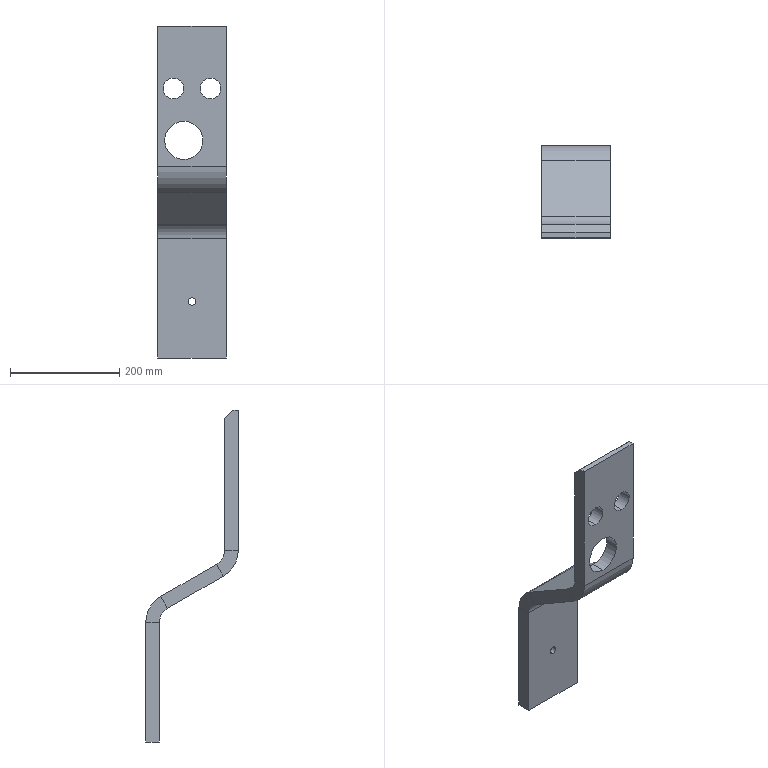Part | SolidWorks | features Chamfer 1, FlatPattern 1, HoleWzd 1, ICE 1, SMBaseFlange 1, SheetMetal 1 | 1 solid | 31 faces | box 126 x 169.5 x 608 mm | volume 1978271 mm3 | plane 19 | cylinder 12 | commonest cylinder face diameters 38 x4 14 x2 60 x2 70 x2 110 x2
STEP:
#1=CARTESIAN_POINT('',(0.,144.5,-397.));
#2=VERTEX_POINT('',#1);
#3=CARTESIAN_POINT('',(0.,144.5,-383.));
#4=VERTEX_POINT('',#3);
#5=CARTESIAN_POINT('',(0.,144.5,-390.));
#6=DIRECTION('',(0.,1.,0.));
#7=DIRECTION('',(0.,0.,1.));
#8=AXIS2_PLACEMENT_3D('',#5,#6,#7);
#9=CIRCLE('',#8,7.);
#10=EDGE_CURVE('',#2,#4,#9,.T.);
#11=ORIENTED_EDGE('',*,*,#10,.F.);
#12=CARTESIAN_POINT('',(0.,169.5,-397.));
#13=VERTEX_POINT('',#12);
#14=CARTESIAN_POINT('',(0.,169.5,-397.));
#15=DIRECTION('',(0.,1.,0.));
#16=VECTOR('',#15,1000.);
#17=LINE('',#14,#16);
#18=EDGE_CURVE('',#2,#13,#17,.T.);
#19=ORIENTED_EDGE('',*,*,#18,.T.);
#20=CARTESIAN_POINT('',(0.,169.5,-383.));
#21=VERTEX_POINT('',#20);
#22=CARTESIAN_POINT('',(0.,169.5,-390.));
#23=DIRECTION('',(0.,1.,0.));
#24=DIRECTION('',(0.,0.,1.));
#25=AXIS2_PLACEMENT_3D('',#22,#23,#24);
#26=CIRCLE('',#25,7.);
#27=EDGE_CURVE('',#13,#21,#26,.T.);
#28=ORIENTED_EDGE('',*,*,#27,.T.);
#29=CARTESIAN_POINT('',(0.,169.5,-383.));
#30=DIRECTION('',(0.,1.,0.));
#31=VECTOR('',#30,1000.);
#32=LINE('',#29,#31);
#33=EDGE_CURVE('',#4,#21,#32,.T.);
#34=ORIENTED_EDGE('',*,*,#33,.F.);
#35=EDGE_LOOP('',(#11,#19,#28,#34));
#36=FACE_OUTER_BOUND('',#35,.T.);
#37=CARTESIAN_POINT('',(0.,169.5,-390.));
#38=DIRECTION('',(0.,1.,0.));
#39=DIRECTION('',(0.,0.,1.));
#40=AXIS2_PLACEMENT_3D('',#37,#38,#39);
#41=CYLINDRICAL_SURFACE('',#40,7.);
#42=ADVANCED_FACE('',(#36),#41,.F.);
#43=CARTESIAN_POINT('',(-15.,25.,-60.));
#44=VERTEX_POINT('',#43);
#45=CARTESIAN_POINT('',(-15.,25.,-130.));
#46=VERTEX_POINT('',#45);
#47=CARTESIAN_POINT('',(-15.,25.,-95.));
#48=DIRECTION('',(0.,-1.,0.));
#49=DIRECTION('',(0.,0.,1.));
#50=AXIS2_PLACEMENT_3D('',#47,#48,#49);
#51=CIRCLE('',#50,35.);
#52=EDGE_CURVE('',#44,#46,#51,.T.);
#53=ORIENTED_EDGE('',*,*,#52,.F.);
#54=CARTESIAN_POINT('',(-15.,0.,-60.));
#55=VERTEX_POINT('',#54);
#56=CARTESIAN_POINT('',(-15.,169.5,-60.));
#57=DIRECTION('',(0.,-1.,0.));
#58=VECTOR('',#57,1000.);
#59=LINE('',#56,#58);
#60=EDGE_CURVE('',#44,#55,#59,.T.);
#61=ORIENTED_EDGE('',*,*,#60,.T.);
#62=CARTESIAN_POINT('',(-15.,0.,-130.));
#63=VERTEX_POINT('',#62);
#64=CARTESIAN_POINT('',(-15.,0.,-95.));
#65=DIRECTION('',(0.,1.,0.));
#66=DIRECTION('',(0.,0.,1.));
#67=AXIS2_PLACEMENT_3D('',#64,#65,#66);
#68=CIRCLE('',#67,35.);
#69=EDGE_CURVE('',#63,#55,#68,.T.);
#70=ORIENTED_EDGE('',*,*,#69,.F.);
#71=CARTESIAN_POINT('',(-15.,169.5,-130.));
#72=DIRECTION('',(0.,-1.,0.));
#73=VECTOR('',#72,1000.);
#74=LINE('',#71,#73);
#75=EDGE_CURVE('',#46,#63,#74,.T.);
#76=ORIENTED_EDGE('',*,*,#75,.F.);
#77=EDGE_LOOP('',(#53,#61,#70,#76));
#78=FACE_OUTER_BOUND('',#77,.T.);
#79=CARTESIAN_POINT('',(-15.,169.5,-95.));
#80=DIRECTION('',(0.,-1.,0.));
#81=DIRECTION('',(0.,0.,-1.));
#82=AXIS2_PLACEMENT_3D('',#79,#80,#81);
#83=CYLINDRICAL_SURFACE('',#82,35.);
#84=ADVANCED_FACE('',(#78),#83,.F.);
#85=CARTESIAN_POINT('',(-34.,25.,19.));
#86=VERTEX_POINT('',#85);
#87=CARTESIAN_POINT('',(-34.,25.,-19.));
#88=VERTEX_POINT('',#87);
#89=CARTESIAN_POINT('',(-34.,25.,0.));
#90=DIRECTION('',(0.,-1.,0.));
#91=DIRECTION('',(0.,0.,1.));
#92=AXIS2_PLACEMENT_3D('',#89,#90,#91);
#93=CIRCLE('',#92,19.);
#94=EDGE_CURVE('',#86,#88,#93,.T.);
#95=ORIENTED_EDGE('',*,*,#94,.F.);
#96=CARTESIAN_POINT('',(-34.,0.,19.));
#97=VERTEX_POINT('',#96);
#98=CARTESIAN_POINT('',(-34.,169.5,19.));
#99=DIRECTION('',(0.,-1.,0.));
#100=VECTOR('',#99,1000.);
#101=LINE('',#98,#100);
#102=EDGE_CURVE('',#86,#97,#101,.T.);
#103=ORIENTED_EDGE('',*,*,#102,.T.);
#104=CARTESIAN_POINT('',(-34.,0.,-19.));
#105=VERTEX_POINT('',#104);
#106=CARTESIAN_POINT('',(-34.,0.,0.));
#107=DIRECTION('',(0.,1.,0.));
#108=DIRECTION('',(0.,0.,1.));
#109=AXIS2_PLACEMENT_3D('',#106,#107,#108);
#110=CIRCLE('',#109,19.);
#111=EDGE_CURVE('',#105,#97,#110,.T.);
#112=ORIENTED_EDGE('',*,*,#111,.F.);
#113=CARTESIAN_POINT('',(-34.,169.5,-19.));
#114=DIRECTION('',(0.,-1.,0.));
#115=VECTOR('',#114,1000.);
#116=LINE('',#113,#115);
#117=EDGE_CURVE('',#88,#105,#116,.T.);
#118=ORIENTED_EDGE('',*,*,#117,.F.);
#119=EDGE_LOOP('',(#95,#103,#112,#118));
#120=FACE_OUTER_BOUND('',#119,.T.);
#121=CARTESIAN_POINT('',(-34.,169.5,0.));
#122=DIRECTION('',(0.,-1.,0.));
#123=DIRECTION('',(0.,0.,-1.));
#124=AXIS2_PLACEMENT_3D('',#121,#122,#123);
#125=CYLINDRICAL_SURFACE('',#124,19.);
#126=ADVANCED_FACE('',(#120),#125,.F.);
#127=CARTESIAN_POINT('',(34.,25.,19.));
#128=VERTEX_POINT('',#127);
#129=CARTESIAN_POINT('',(34.,25.,-19.));
#130=VERTEX_POINT('',#129);
#131=CARTESIAN_POINT('',(34.,25.,0.));
#132=DIRECTION('',(0.,-1.,0.));
#133=DIRECTION('',(0.,0.,1.));
#134=AXIS2_PLACEMENT_3D('',#131,#132,#133);
#135=CIRCLE('',#134,19.);
#136=EDGE_CURVE('',#128,#130,#135,.T.);
#137=ORIENTED_EDGE('',*,*,#136,.F.);
#138=CARTESIAN_POINT('',(34.,0.,19.));
#139=VERTEX_POINT('',#138);
#140=CARTESIAN_POINT('',(34.,169.5,19.));
#141=DIRECTION('',(0.,-1.,0.));
#142=VECTOR('',#141,1000.);
#143=LINE('',#140,#142);
#144=EDGE_CURVE('',#128,#139,#143,.T.);
#145=ORIENTED_EDGE('',*,*,#144,.T.);
#146=CARTESIAN_POINT('',(34.,0.,-19.));
#147=VERTEX_POINT('',#146);
#148=CARTESIAN_POINT('',(34.,0.,0.));
#149=DIRECTION('',(0.,1.,0.));
#150=DIRECTION('',(0.,0.,1.));
#151=AXIS2_PLACEMENT_3D('',#148,#149,#150);
#152=CIRCLE('',#151,19.);
#153=EDGE_CURVE('',#147,#139,#152,.T.);
#154=ORIENTED_EDGE('',*,*,#153,.F.);
#155=CARTESIAN_POINT('',(34.,169.5,-19.));
#156=DIRECTION('',(0.,-1.,0.));
#157=VECTOR('',#156,1000.);
#158=LINE('',#155,#157);
#159=EDGE_CURVE('',#130,#147,#158,.T.);
#160=ORIENTED_EDGE('',*,*,#159,.F.);
#161=EDGE_LOOP('',(#137,#145,#154,#160));
#162=FACE_OUTER_BOUND('',#161,.T.);
#163=CARTESIAN_POINT('',(34.,169.5,0.));
#164=DIRECTION('',(0.,-1.,0.));
#165=DIRECTION('',(0.,0.,-1.));
#166=AXIS2_PLACEMENT_3D('',#163,#164,#165);
#167=CYLINDRICAL_SURFACE('',#166,19.);
#168=ADVANCED_FACE('',(#162),#167,.F.);
#169=CARTESIAN_POINT('',(-34.,25.,0.));
#170=DIRECTION('',(0.,-1.,0.));
#171=DIRECTION('',(0.,0.,1.));
#172=AXIS2_PLACEMENT_3D('',#169,#170,#171);
#173=CIRCLE('',#172,19.);
#174=EDGE_CURVE('',#88,#86,#173,.T.);
#175=ORIENTED_EDGE('',*,*,#174,.T.);
#176=ORIENTED_EDGE('',*,*,#94,.T.);
#177=EDGE_LOOP('',(#175,#176));
#178=FACE_BOUND('',#177,.T.);
#179=CARTESIAN_POINT('',(-63.,25.,99.5));
#180=VERTEX_POINT('',#179);
#181=CARTESIAN_POINT('',(-63.,25.,-142.179));
#182=VERTEX_POINT('',#181);
#183=CARTESIAN_POINT('',(-63.,25.,114.5));
#184=DIRECTION('',(0.,0.,-1.));
#185=VECTOR('',#184,1000.);
#186=LINE('',#183,#185);
#187=EDGE_CURVE('',#180,#182,#186,.T.);
#188=ORIENTED_EDGE('',*,*,#187,.F.);
#189=CARTESIAN_POINT('',(63.,25.,99.5));
#190=VERTEX_POINT('',#189);
#191=CARTESIAN_POINT('',(63.,25.,99.5));
#192=DIRECTION('',(1.,0.,0.));
#193=VECTOR('',#192,1000.);
#194=LINE('',#191,#193);
#195=EDGE_CURVE('',#180,#190,#194,.T.);
#196=ORIENTED_EDGE('',*,*,#195,.T.);
#197=CARTESIAN_POINT('',(63.,25.,-142.179));
#198=VERTEX_POINT('',#197);
#199=CARTESIAN_POINT('',(63.,25.,114.5));
#200=DIRECTION('',(0.,0.,-1.));
#201=VECTOR('',#200,1000.);
#202=LINE('',#199,#201);
#203=EDGE_CURVE('',#190,#198,#202,.T.);
#204=ORIENTED_EDGE('',*,*,#203,.T.);
#205=CARTESIAN_POINT('',(63.,25.,-142.179));
#206=DIRECTION('',(-1.,0.,0.));
#207=VECTOR('',#206,1000.);
#208=LINE('',#205,#207);
#209=EDGE_CURVE('',#198,#182,#208,.T.);
#210=ORIENTED_EDGE('',*,*,#209,.T.);
#211=EDGE_LOOP('',(#188,#196,#204,#210));
#212=FACE_OUTER_BOUND('',#211,.T.);
#213=CARTESIAN_POINT('',(34.,25.,0.));
#214=DIRECTION('',(0.,-1.,0.));
#215=DIRECTION('',(0.,0.,1.));
#216=AXIS2_PLACEMENT_3D('',#213,#214,#215);
#217=CIRCLE('',#216,19.);
#218=EDGE_CURVE('',#130,#128,#217,.T.);
#219=ORIENTED_EDGE('',*,*,#218,.T.);
#220=ORIENTED_EDGE('',*,*,#136,.T.);
#221=EDGE_LOOP('',(#219,#220));
#222=FACE_BOUND('',#221,.T.);
#223=CARTESIAN_POINT('',(-15.,25.,-95.));
#224=DIRECTION('',(0.,-1.,0.));
#225=DIRECTION('',(0.,0.,1.));
#226=AXIS2_PLACEMENT_3D('',#223,#224,#225);
#227=CIRCLE('',#226,35.);
#228=EDGE_CURVE('',#46,#44,#227,.T.);
#229=ORIENTED_EDGE('',*,*,#228,.T.);
#230=ORIENTED_EDGE('',*,*,#52,.T.);
#231=EDGE_LOOP('',(#229,#230));
#232=FACE_BOUND('',#231,.T.);
#233=CARTESIAN_POINT('',(63.,25.,114.5));
#234=DIRECTION('',(0.,1.,0.));
#235=DIRECTION('',(0.,0.,1.));
#236=AXIS2_PLACEMENT_3D('',#233,#234,#235);
#237=PLANE('',#236);
#238=ADVANCED_FACE('',(#178,#212,#222,#232),#237,.T.);
#239=ORIENTED_EDGE('',*,*,#111,.T.);
#240=CARTESIAN_POINT('',(-34.,0.,0.));
#241=DIRECTION('',(0.,1.,0.));
#242=DIRECTION('',(0.,0.,1.));
#243=AXIS2_PLACEMENT_3D('',#240,#241,#242);
#244=CIRCLE('',#243,19.);
#245=EDGE_CURVE('',#97,#105,#244,.T.);
#246=ORIENTED_EDGE('',*,*,#245,.T.);
#247=EDGE_LOOP('',(#239,#246));
#248=FACE_BOUND('',#247,.T.);
#249=CARTESIAN_POINT('',(-63.,0.,114.5));
#250=VERTEX_POINT('',#249);
#251=CARTESIAN_POINT('',(-63.,0.,-142.179));
#252=VERTEX_POINT('',#251);
#253=CARTESIAN_POINT('',(-63.,0.,114.5));
#254=DIRECTION('',(0.,0.,-1.));
#255=VECTOR('',#254,1000.);
#256=LINE('',#253,#255);
#257=EDGE_CURVE('',#250,#252,#256,.T.);
#258=ORIENTED_EDGE('',*,*,#257,.T.);
#259=CARTESIAN_POINT('',(63.,0.,-142.179));
#260=VERTEX_POINT('',#259);
#261=CARTESIAN_POINT('',(63.,0.,-142.179));
#262=DIRECTION('',(-1.,0.,0.));
#263=VECTOR('',#262,1000.);
#264=LINE('',#261,#263);
#265=EDGE_CURVE('',#260,#252,#264,.T.);
#266=ORIENTED_EDGE('',*,*,#265,.F.);
#267=CARTESIAN_POINT('',(63.,0.,114.5));
#268=VERTEX_POINT('',#267);
#269=CARTESIAN_POINT('',(63.,0.,114.5));
#270=DIRECTION('',(0.,0.,-1.));
#271=VECTOR('',#270,1000.);
#272=LINE('',#269,#271);
#273=EDGE_CURVE('',#268,#260,#272,.T.);
#274=ORIENTED_EDGE('',*,*,#273,.F.);
#275=CARTESIAN_POINT('',(63.,0.,114.5));
#276=DIRECTION('',(-1.,0.,0.));
#277=VECTOR('',#276,1000.);
#278=LINE('',#275,#277);
#279=EDGE_CURVE('',#268,#250,#278,.T.);
#280=ORIENTED_EDGE('',*,*,#279,.T.);
#281=EDGE_LOOP('',(#258,#266,#274,#280));
#282=FACE_OUTER_BOUND('',#281,.T.);
#283=ORIENTED_EDGE('',*,*,#153,.T.);
#284=CARTESIAN_POINT('',(34.,0.,0.));
#285=DIRECTION('',(0.,1.,0.));
#286=DIRECTION('',(0.,0.,1.));
#287=AXIS2_PLACEMENT_3D('',#284,#285,#286);
#288=CIRCLE('',#287,19.);
#289=EDGE_CURVE('',#139,#147,#288,.T.);
#290=ORIENTED_EDGE('',*,*,#289,.T.);
#291=EDGE_LOOP('',(#283,#290));
#292=FACE_BOUND('',#291,.T.);
#293=ORIENTED_EDGE('',*,*,#69,.T.);
#294=CARTESIAN_POINT('',(-15.,0.,-95.));
#295=DIRECTION('',(0.,1.,0.));
#296=DIRECTION('',(0.,0.,1.));
#297=AXIS2_PLACEMENT_3D('',#294,#295,#296);
#298=CIRCLE('',#297,35.);
#299=EDGE_CURVE('',#55,#63,#298,.T.);
#300=ORIENTED_EDGE('',*,*,#299,.T.);
#301=EDGE_LOOP('',(#293,#300));
#302=FACE_BOUND('',#301,.T.);
#303=CARTESIAN_POINT('',(63.,0.,114.5));
#304=DIRECTION('',(0.,1.,0.));
#305=DIRECTION('',(0.,0.,1.));
#306=AXIS2_PLACEMENT_3D('',#303,#304,#305);
#307=PLANE('',#306);
#308=ADVANCED_FACE('',(#248,#282,#292,#302),#307,.F.);
#309=CARTESIAN_POINT('',(63.,40.,-168.16));
#310=VERTEX_POINT('',#309);
#311=CARTESIAN_POINT('',(63.,27.5,-189.811));
#312=VERTEX_POINT('',#311);
#313=CARTESIAN_POINT('',(63.,40.,-168.16));
#314=DIRECTION('',(0.,-0.5,-0.866));
#315=VECTOR('',#314,1000.);
#316=LINE('',#313,#315);
#317=EDGE_CURVE('',#310,#312,#316,.T.);
#318=ORIENTED_EDGE('',*,*,#317,.F.);
#319=CARTESIAN_POINT('',(63.,55.,-142.179));
#320=DIRECTION('',(1.,0.,0.));
#321=DIRECTION('',(0.,0.,1.));
#322=AXIS2_PLACEMENT_3D('',#319,#320,#321);
#323=CIRCLE('',#322,30.);
#324=EDGE_CURVE('',#198,#310,#323,.T.);
#325=ORIENTED_EDGE('',*,*,#324,.F.);
#326=CARTESIAN_POINT('',(63.,0.,-142.179));
#327=DIRECTION('',(0.,1.,0.));
#328=VECTOR('',#327,1000.);
#329=LINE('',#326,#328);
#330=EDGE_CURVE('',#260,#198,#329,.T.);
#331=ORIENTED_EDGE('',*,*,#330,.F.);
#332=CARTESIAN_POINT('',(63.,55.,-142.179));
#333=DIRECTION('',(1.,0.,0.));
#334=DIRECTION('',(0.,0.,-1.));
#335=AXIS2_PLACEMENT_3D('',#332,#333,#334);
#336=CIRCLE('',#335,55.);
#337=EDGE_CURVE('',#260,#312,#336,.T.);
#338=ORIENTED_EDGE('',*,*,#337,.T.);
#339=EDGE_LOOP('',(#318,#325,#331,#338));
#340=FACE_OUTER_BOUND('',#339,.T.);
#341=CARTESIAN_POINT('',(63.,40.,-168.16));
#342=DIRECTION('',(1.,0.,0.));
#343=DIRECTION('',(0.,0.,-1.));
#344=AXIS2_PLACEMENT_3D('',#341,#342,#343);
#345=PLANE('',#344);
#346=ADVANCED_FACE('',(#340),#345,.T.);
#347=CARTESIAN_POINT('',(63.,142.,-227.05));
#348=VERTEX_POINT('',#347);
#349=CARTESIAN_POINT('',(63.,25.,-159.5));
#350=DIRECTION('',(0.,0.866,-0.5));
#351=VECTOR('',#350,1000.);
#352=LINE('',#349,#351);
#353=EDGE_CURVE('',#310,#348,#352,.T.);
#354=ORIENTED_EDGE('',*,*,#353,.F.);
#355=ORIENTED_EDGE('',*,*,#317,.T.);
#356=CARTESIAN_POINT('',(63.,129.5,-248.701));
#357=VERTEX_POINT('',#356);
#358=CARTESIAN_POINT('',(63.,12.5,-181.151));
#359=DIRECTION('',(0.,0.866,-0.5));
#360=VECTOR('',#359,1000.);
#361=LINE('',#358,#360);
#362=EDGE_CURVE('',#312,#357,#361,.T.);
#363=ORIENTED_EDGE('',*,*,#362,.T.);
#364=CARTESIAN_POINT('',(63.,129.5,-248.701));
#365=DIRECTION('',(0.,0.5,0.866));
#366=VECTOR('',#365,1000.);
#367=LINE('',#364,#366);
#368=EDGE_CURVE('',#357,#348,#367,.T.);
#369=ORIENTED_EDGE('',*,*,#368,.T.);
#370=EDGE_LOOP('',(#354,#355,#363,#369));
#371=FACE_OUTER_BOUND('',#370,.T.);
#372=CARTESIAN_POINT('',(63.,0.,-142.179));
#373=DIRECTION('',(1.,0.,0.));
#374=DIRECTION('',(0.,0.,-1.));
#375=AXIS2_PLACEMENT_3D('',#372,#373,#374);
#376=PLANE('',#375);
#377=ADVANCED_FACE('',(#371),#376,.T.);
#378=CARTESIAN_POINT('',(-63.,25.,-142.179));
#379=DIRECTION('',(0.,-1.,0.));
#380=VECTOR('',#379,1000.);
#381=LINE('',#378,#380);
#382=EDGE_CURVE('',#182,#252,#381,.T.);
#383=ORIENTED_EDGE('',*,*,#382,.F.);
#384=CARTESIAN_POINT('',(-63.,40.,-168.16));
#385=VERTEX_POINT('',#384);
#386=CARTESIAN_POINT('',(-63.,55.,-142.179));
#387=DIRECTION('',(1.,0.,0.));
#388=DIRECTION('',(0.,0.,1.));
#389=AXIS2_PLACEMENT_3D('',#386,#387,#388);
#390=CIRCLE('',#389,30.);
#391=EDGE_CURVE('',#182,#385,#390,.T.);
#392=ORIENTED_EDGE('',*,*,#391,.T.);
#393=CARTESIAN_POINT('',(-63.,27.5,-189.811));
#394=VERTEX_POINT('',#393);
#395=CARTESIAN_POINT('',(-63.,27.5,-189.811));
#396=DIRECTION('',(0.,0.5,0.866));
#397=VECTOR('',#396,1000.);
#398=LINE('',#395,#397);
#399=EDGE_CURVE('',#394,#385,#398,.T.);
#400=ORIENTED_EDGE('',*,*,#399,.F.);
#401=CARTESIAN_POINT('',(-63.,55.,-142.179));
#402=DIRECTION('',(1.,0.,0.));
#403=DIRECTION('',(0.,0.,-1.));
#404=AXIS2_PLACEMENT_3D('',#401,#402,#403);
#405=CIRCLE('',#404,55.);
#406=EDGE_CURVE('',#252,#394,#405,.T.);
#407=ORIENTED_EDGE('',*,*,#406,.F.);
#408=EDGE_LOOP('',(#383,#392,#400,#407));
#409=FACE_OUTER_BOUND('',#408,.T.);
#410=CARTESIAN_POINT('',(-63.,25.,-142.179));
#411=DIRECTION('',(-1.,0.,0.));
#412=DIRECTION('',(0.,0.,1.));
#413=AXIS2_PLACEMENT_3D('',#410,#411,#412);
#414=PLANE('',#413);
#415=ADVANCED_FACE('',(#409),#414,.T.);
#416=CARTESIAN_POINT('',(-63.,10.,114.5));
#417=VERTEX_POINT('',#416);
#418=CARTESIAN_POINT('',(-63.,0.,114.5));
#419=DIRECTION('',(0.,1.,0.));
#420=VECTOR('',#419,1000.);
#421=LINE('',#418,#420);
#422=EDGE_CURVE('',#250,#417,#421,.T.);
#423=ORIENTED_EDGE('',*,*,#422,.T.);
#424=CARTESIAN_POINT('',(-63.,170.905,-46.405));
#425=DIRECTION('',(0.,0.7071,-0.7071));
#426=VECTOR('',#425,1000.);
#427=LINE('',#424,#426);
#428=EDGE_CURVE('',#417,#180,#427,.T.);
#429=ORIENTED_EDGE('',*,*,#428,.T.);
#430=ORIENTED_EDGE('',*,*,#187,.T.);
#431=ORIENTED_EDGE('',*,*,#382,.T.);
#432=ORIENTED_EDGE('',*,*,#257,.F.);
#433=EDGE_LOOP('',(#423,#429,#430,#431,#432));
#434=FACE_OUTER_BOUND('',#433,.T.);
#435=CARTESIAN_POINT('',(-63.,27.5,-189.811));
#436=DIRECTION('',(-1.,0.,0.));
#437=DIRECTION('',(0.,0.,1.));
#438=AXIS2_PLACEMENT_3D('',#435,#436,#437);
#439=PLANE('',#438);
#440=ADVANCED_FACE('',(#434),#439,.T.);
#441=CARTESIAN_POINT('',(63.,169.5,-274.681));
#442=VERTEX_POINT('',#441);
#443=CARTESIAN_POINT('',(63.,144.5,-274.681));
#444=VERTEX_POINT('',#443);
#445=CARTESIAN_POINT('',(63.,169.5,-274.681));
#446=DIRECTION('',(0.,-1.,0.));
#447=VECTOR('',#446,1000.);
#448=LINE('',#445,#447);
#449=EDGE_CURVE('',#442,#444,#448,.T.);
#450=ORIENTED_EDGE('',*,*,#449,.F.);
#451=CARTESIAN_POINT('',(63.,114.5,-274.681));
#452=DIRECTION('',(-1.,0.,0.));
#453=DIRECTION('',(0.,0.,-1.));
#454=AXIS2_PLACEMENT_3D('',#451,#452,#453);
#455=CIRCLE('',#454,55.);
#456=EDGE_CURVE('',#348,#442,#455,.T.);
#457=ORIENTED_EDGE('',*,*,#456,.F.);
#458=ORIENTED_EDGE('',*,*,#368,.F.);
#459=CARTESIAN_POINT('',(63.,114.5,-274.681));
#460=DIRECTION('',(-1.,0.,0.));
#461=DIRECTION('',(0.,0.,-1.));
#462=AXIS2_PLACEMENT_3D('',#459,#460,#461);
#463=CIRCLE('',#462,30.);
#464=EDGE_CURVE('',#357,#444,#463,.T.);
#465=ORIENTED_EDGE('',*,*,#464,.T.);
#466=EDGE_LOOP('',(#450,#457,#458,#465));
#467=FACE_OUTER_BOUND('',#466,.T.);
#468=CARTESIAN_POINT('',(63.,169.5,-274.681));
#469=DIRECTION('',(1.,0.,0.));
#470=DIRECTION('',(0.,0.,-1.));
#471=AXIS2_PLACEMENT_3D('',#468,#469,#470);
#472=PLANE('',#471);
#473=ADVANCED_FACE('',(#467),#472,.T.);
#474=CARTESIAN_POINT('',(63.,169.5,-493.5));
#475=VERTEX_POINT('',#474);
#476=CARTESIAN_POINT('',(63.,169.5,-242.927));
#477=DIRECTION('',(0.,0.,-1.));
#478=VECTOR('',#477,1000.);
#479=LINE('',#476,#478);
#480=EDGE_CURVE('',#442,#475,#479,.T.);
#481=ORIENTED_EDGE('',*,*,#480,.F.);
#482=ORIENTED_EDGE('',*,*,#449,.T.);
#483=CARTESIAN_POINT('',(63.,144.5,-493.5));
#484=VERTEX_POINT('',#483);
#485=CARTESIAN_POINT('',(63.,144.5,-242.927));
#486=DIRECTION('',(0.,0.,-1.));
#487=VECTOR('',#486,1000.);
#488=LINE('',#485,#487);
#489=EDGE_CURVE('',#444,#484,#488,.T.);
#490=ORIENTED_EDGE('',*,*,#489,.T.);
#491=CARTESIAN_POINT('',(63.,169.5,-493.5));
#492=DIRECTION('',(0.,-1.,0.));
#493=VECTOR('',#492,1000.);
#494=LINE('',#491,#493);
#495=EDGE_CURVE('',#475,#484,#494,.T.);
#496=ORIENTED_EDGE('',*,*,#495,.F.);
#497=EDGE_LOOP('',(#481,#482,#490,#496));
#498=FACE_OUTER_BOUND('',#497,.T.);
#499=CARTESIAN_POINT('',(63.,129.5,-248.701));
#500=DIRECTION('',(1.,0.,0.));
#501=DIRECTION('',(0.,0.,-1.));
#502=AXIS2_PLACEMENT_3D('',#499,#500,#501);
#503=PLANE('',#502);
#504=ADVANCED_FACE('',(#498),#503,.T.);
#505=CARTESIAN_POINT('',(-63.,142.,-227.05));
#506=VERTEX_POINT('',#505);
#507=CARTESIAN_POINT('',(-63.,129.5,-248.701));
#508=VERTEX_POINT('',#507);
#509=CARTESIAN_POINT('',(-63.,142.,-227.05));
#510=DIRECTION('',(0.,-0.5,-0.866));
#511=VECTOR('',#510,1000.);
#512=LINE('',#509,#511);
#513=EDGE_CURVE('',#506,#508,#512,.T.);
#514=ORIENTED_EDGE('',*,*,#513,.F.);
#515=CARTESIAN_POINT('',(-63.,169.5,-274.681));
#516=VERTEX_POINT('',#515);
#517=CARTESIAN_POINT('',(-63.,114.5,-274.681));
#518=DIRECTION('',(-1.,0.,0.));
#519=DIRECTION('',(0.,0.,-1.));
#520=AXIS2_PLACEMENT_3D('',#517,#518,#519);
#521=CIRCLE('',#520,55.);
#522=EDGE_CURVE('',#506,#516,#521,.T.);
#523=ORIENTED_EDGE('',*,*,#522,.T.);
#524=CARTESIAN_POINT('',(-63.,144.5,-274.681));
#525=VERTEX_POINT('',#524);
#526=CARTESIAN_POINT('',(-63.,144.5,-274.681));
#527=DIRECTION('',(0.,1.,0.));
#528=VECTOR('',#527,1000.);
#529=LINE('',#526,#528);
#530=EDGE_CURVE('',#525,#516,#529,.T.);
#531=ORIENTED_EDGE('',*,*,#530,.F.);
#532=CARTESIAN_POINT('',(-63.,114.5,-274.681));
#533=DIRECTION('',(-1.,0.,0.));
#534=DIRECTION('',(0.,0.,-1.));
#535=AXIS2_PLACEMENT_3D('',#532,#533,#534);
#536=CIRCLE('',#535,30.);
#537=EDGE_CURVE('',#508,#525,#536,.T.);
#538=ORIENTED_EDGE('',*,*,#537,.F.);
#539=EDGE_LOOP('',(#514,#523,#531,#538));
#540=FACE_OUTER_BOUND('',#539,.T.);
#541=CARTESIAN_POINT('',(-63.,142.,-227.05));
#542=DIRECTION('',(-1.,0.,0.));
#543=DIRECTION('',(0.,0.,1.));
#544=AXIS2_PLACEMENT_3D('',#541,#542,#543);
#545=PLANE('',#544);
#546=ADVANCED_FACE('',(#540),#545,.T.);
#547=CARTESIAN_POINT('',(-63.,25.,-159.5));
#548=DIRECTION('',(0.,0.866,-0.5));
#549=VECTOR('',#548,1000.);
#550=LINE('',#547,#549);
#551=EDGE_CURVE('',#385,#506,#550,.T.);
#552=ORIENTED_EDGE('',*,*,#551,.T.);
#553=ORIENTED_EDGE('',*,*,#513,.T.);
#554=CARTESIAN_POINT('',(-63.,12.5,-181.151));
#555=DIRECTION('',(0.,0.866,-0.5));
#556=VECTOR('',#555,1000.);
#557=LINE('',#554,#556);
#558=EDGE_CURVE('',#394,#508,#557,.T.);
#559=ORIENTED_EDGE('',*,*,#558,.F.);
#560=ORIENTED_EDGE('',*,*,#399,.T.);
#561=EDGE_LOOP('',(#552,#553,#559,#560));
#562=FACE_OUTER_BOUND('',#561,.T.);
#563=CARTESIAN_POINT('',(-63.,144.5,-274.681));
#564=DIRECTION('',(-1.,0.,0.));
#565=DIRECTION('',(0.,0.,1.));
#566=AXIS2_PLACEMENT_3D('',#563,#564,#565);
#567=PLANE('',#566);
#568=ADVANCED_FACE('',(#562),#567,.T.);
#569=CARTESIAN_POINT('',(0.,144.5,-390.));
#570=DIRECTION('',(0.,1.,0.));
#571=DIRECTION('',(0.,0.,1.));
#572=AXIS2_PLACEMENT_3D('',#569,#570,#571);
#573=CIRCLE('',#572,7.);
#574=EDGE_CURVE('',#4,#2,#573,.T.);
#575=ORIENTED_EDGE('',*,*,#574,.T.);
#576=ORIENTED_EDGE('',*,*,#10,.T.);
#577=EDGE_LOOP('',(#575,#576));
#578=FACE_BOUND('',#577,.T.);
#579=CARTESIAN_POINT('',(-63.,144.5,-493.5));
#580=VERTEX_POINT('',#579);
#581=CARTESIAN_POINT('',(-63.,144.5,-242.927));
#582=DIRECTION('',(0.,0.,-1.));
#583=VECTOR('',#582,1000.);
#584=LINE('',#581,#583);
#585=EDGE_CURVE('',#525,#580,#584,.T.);
#586=ORIENTED_EDGE('',*,*,#585,.T.);
#587=CARTESIAN_POINT('',(63.,144.5,-493.5));
#588=DIRECTION('',(-1.,0.,0.));
#589=VECTOR('',#588,1000.);
#590=LINE('',#587,#589);
#591=EDGE_CURVE('',#484,#580,#590,.T.);
#592=ORIENTED_EDGE('',*,*,#591,.F.);
#593=ORIENTED_EDGE('',*,*,#489,.F.);
#594=CARTESIAN_POINT('',(63.,144.5,-274.681));
#595=DIRECTION('',(-1.,0.,0.));
#596=VECTOR('',#595,1000.);
#597=LINE('',#594,#596);
#598=EDGE_CURVE('',#444,#525,#597,.T.);
#599=ORIENTED_EDGE('',*,*,#598,.T.);
#600=EDGE_LOOP('',(#586,#592,#593,#599));
#601=FACE_OUTER_BOUND('',#600,.T.);
#602=CARTESIAN_POINT('',(63.,144.5,-242.927));
#603=DIRECTION('',(0.,1.,0.));
#604=DIRECTION('',(0.,0.,1.));
#605=AXIS2_PLACEMENT_3D('',#602,#603,#604);
#606=PLANE('',#605);
#607=ADVANCED_FACE('',(#578,#601),#606,.F.);
#608=CARTESIAN_POINT('',(-63.,169.5,-493.5));
#609=VERTEX_POINT('',#608);
#610=CARTESIAN_POINT('',(-63.,169.5,-493.5));
#611=DIRECTION('',(0.,-1.,0.));
#612=VECTOR('',#611,1000.);
#613=LINE('',#610,#612);
#614=EDGE_CURVE('',#609,#580,#613,.T.);
#615=ORIENTED_EDGE('',*,*,#614,.F.);
#616=CARTESIAN_POINT('',(63.,169.5,-493.5));
#617=DIRECTION('',(-1.,0.,0.));
#618=VECTOR('',#617,1000.);
#619=LINE('',#616,#618);
#620=EDGE_CURVE('',#475,#609,#619,.T.);
#621=ORIENTED_EDGE('',*,*,#620,.F.);
#622=ORIENTED_EDGE('',*,*,#495,.T.);
#623=ORIENTED_EDGE('',*,*,#591,.T.);
#624=EDGE_LOOP('',(#615,#621,#622,#623));
#625=FACE_OUTER_BOUND('',#624,.T.);
#626=CARTESIAN_POINT('',(63.,169.5,-493.5));
#627=DIRECTION('',(0.,0.,-1.));
#628=DIRECTION('',(-1.,0.,0.));
#629=AXIS2_PLACEMENT_3D('',#626,#627,#628);
#630=PLANE('',#629);
#631=ADVANCED_FACE('',(#625),#630,.T.);
#632=CARTESIAN_POINT('',(0.,169.5,-390.));
#633=DIRECTION('',(0.,1.,0.));
#634=DIRECTION('',(0.,0.,1.));
#635=AXIS2_PLACEMENT_3D('',#632,#633,#634);
#636=CIRCLE('',#635,7.);
#637=EDGE_CURVE('',#21,#13,#636,.T.);
#638=ORIENTED_EDGE('',*,*,#637,.F.);
#639=ORIENTED_EDGE('',*,*,#27,.F.);
#640=EDGE_LOOP('',(#638,#639));
#641=FACE_BOUND('',#640,.T.);
#642=CARTESIAN_POINT('',(-63.,169.5,-242.927));
#643=DIRECTION('',(0.,0.,-1.));
#644=VECTOR('',#643,1000.);
#645=LINE('',#642,#644);
#646=EDGE_CURVE('',#516,#609,#645,.T.);
#647=ORIENTED_EDGE('',*,*,#646,.F.);
#648=CARTESIAN_POINT('',(63.,169.5,-274.681));
#649=DIRECTION('',(-1.,0.,0.));
#650=VECTOR('',#649,1000.);
#651=LINE('',#648,#650);
#652=EDGE_CURVE('',#442,#516,#651,.T.);
#653=ORIENTED_EDGE('',*,*,#652,.F.);
#654=ORIENTED_EDGE('',*,*,#480,.T.);
#655=ORIENTED_EDGE('',*,*,#620,.T.);
#656=EDGE_LOOP('',(#647,#653,#654,#655));
#657=FACE_OUTER_BOUND('',#656,.T.);
#658=CARTESIAN_POINT('',(63.,169.5,-242.927));
#659=DIRECTION('',(0.,1.,0.));
#660=DIRECTION('',(0.,0.,1.));
#661=AXIS2_PLACEMENT_3D('',#658,#659,#660);
#662=PLANE('',#661);
#663=ADVANCED_FACE('',(#641,#657),#662,.T.);
#664=ORIENTED_EDGE('',*,*,#522,.F.);
#665=CARTESIAN_POINT('',(63.,142.,-227.05));
#666=DIRECTION('',(-1.,0.,0.));
#667=VECTOR('',#666,1000.);
#668=LINE('',#665,#667);
#669=EDGE_CURVE('',#348,#506,#668,.T.);
#670=ORIENTED_EDGE('',*,*,#669,.F.);
#671=ORIENTED_EDGE('',*,*,#456,.T.);
#672=ORIENTED_EDGE('',*,*,#652,.T.);
#673=EDGE_LOOP('',(#664,#670,#671,#672));
#674=FACE_OUTER_BOUND('',#673,.T.);
#675=CARTESIAN_POINT('',(63.,114.5,-274.681));
#676=DIRECTION('',(-1.,0.,0.));
#677=DIRECTION('',(0.,0.,1.));
#678=AXIS2_PLACEMENT_3D('',#675,#676,#677);
#679=CYLINDRICAL_SURFACE('',#678,55.);
#680=ADVANCED_FACE('',(#674),#679,.T.);
#681=ORIENTED_EDGE('',*,*,#551,.F.);
#682=CARTESIAN_POINT('',(63.,40.,-168.16));
#683=DIRECTION('',(-1.,0.,0.));
#684=VECTOR('',#683,1000.);
#685=LINE('',#682,#684);
#686=EDGE_CURVE('',#310,#385,#685,.T.);
#687=ORIENTED_EDGE('',*,*,#686,.F.);
#688=ORIENTED_EDGE('',*,*,#353,.T.);
#689=ORIENTED_EDGE('',*,*,#669,.T.);
#690=EDGE_LOOP('',(#681,#687,#688,#689));
#691=FACE_OUTER_BOUND('',#690,.T.);
#692=CARTESIAN_POINT('',(63.,25.,-159.5));
#693=DIRECTION('',(0.,0.5,0.866));
#694=DIRECTION('',(0.,-0.866,0.5));
#695=AXIS2_PLACEMENT_3D('',#692,#693,#694);
#696=PLANE('',#695);
#697=ADVANCED_FACE('',(#691),#696,.T.);
#698=ORIENTED_EDGE('',*,*,#391,.F.);
#699=ORIENTED_EDGE('',*,*,#209,.F.);
#700=ORIENTED_EDGE('',*,*,#324,.T.);
#701=ORIENTED_EDGE('',*,*,#686,.T.);
#702=EDGE_LOOP('',(#698,#699,#700,#701));
#703=FACE_OUTER_BOUND('',#702,.T.);
#704=CARTESIAN_POINT('',(63.,55.,-142.179));
#705=DIRECTION('',(-1.,0.,0.));
#706=DIRECTION('',(0.,0.,1.));
#707=AXIS2_PLACEMENT_3D('',#704,#705,#706);
#708=CYLINDRICAL_SURFACE('',#707,30.);
#709=ADVANCED_FACE('',(#703),#708,.F.);
#710=CARTESIAN_POINT('',(63.,10.,114.5));
#711=VERTEX_POINT('',#710);
#712=CARTESIAN_POINT('',(63.,0.,114.5));
#713=DIRECTION('',(0.,1.,0.));
#714=VECTOR('',#713,1000.);
#715=LINE('',#712,#714);
#716=EDGE_CURVE('',#268,#711,#715,.T.);
#717=ORIENTED_EDGE('',*,*,#716,.T.);
#718=CARTESIAN_POINT('',(63.,10.,114.5));
#719=DIRECTION('',(-1.,0.,0.));
#720=VECTOR('',#719,1000.);
#721=LINE('',#718,#720);
#722=EDGE_CURVE('',#711,#417,#721,.T.);
#723=ORIENTED_EDGE('',*,*,#722,.T.);
#724=ORIENTED_EDGE('',*,*,#422,.F.);
#725=ORIENTED_EDGE('',*,*,#279,.F.);
#726=EDGE_LOOP('',(#717,#723,#724,#725));
#727=FACE_OUTER_BOUND('',#726,.T.);
#728=CARTESIAN_POINT('',(63.,0.,114.5));
#729=DIRECTION('',(0.,0.,1.));
#730=DIRECTION('',(1.,0.,0.));
#731=AXIS2_PLACEMENT_3D('',#728,#729,#730);
#732=PLANE('',#731);
#733=ADVANCED_FACE('',(#727),#732,.T.);
#734=ORIENTED_EDGE('',*,*,#406,.T.);
#735=CARTESIAN_POINT('',(63.,27.5,-189.811));
#736=DIRECTION('',(-1.,0.,0.));
#737=VECTOR('',#736,1000.);
#738=LINE('',#735,#737);
#739=EDGE_CURVE('',#312,#394,#738,.T.);
#740=ORIENTED_EDGE('',*,*,#739,.F.);
#741=ORIENTED_EDGE('',*,*,#337,.F.);
#742=ORIENTED_EDGE('',*,*,#265,.T.);
#743=EDGE_LOOP('',(#734,#740,#741,#742));
#744=FACE_OUTER_BOUND('',#743,.T.);
#745=CARTESIAN_POINT('',(63.,55.,-142.179));
#746=DIRECTION('',(-1.,0.,0.));
#747=DIRECTION('',(0.,0.,1.));
#748=AXIS2_PLACEMENT_3D('',#745,#746,#747);
#749=CYLINDRICAL_SURFACE('',#748,55.);
#750=ADVANCED_FACE('',(#744),#749,.T.);
#751=ORIENTED_EDGE('',*,*,#558,.T.);
#752=CARTESIAN_POINT('',(63.,129.5,-248.701));
#753=DIRECTION('',(-1.,0.,0.));
#754=VECTOR('',#753,1000.);
#755=LINE('',#752,#754);
#756=EDGE_CURVE('',#357,#508,#755,.T.);
#757=ORIENTED_EDGE('',*,*,#756,.F.);
#758=ORIENTED_EDGE('',*,*,#362,.F.);
#759=ORIENTED_EDGE('',*,*,#739,.T.);
#760=EDGE_LOOP('',(#751,#757,#758,#759));
#761=FACE_OUTER_BOUND('',#760,.T.);
#762=CARTESIAN_POINT('',(63.,12.5,-181.151));
#763=DIRECTION('',(0.,0.5,0.866));
#764=DIRECTION('',(0.,-0.866,0.5));
#765=AXIS2_PLACEMENT_3D('',#762,#763,#764);
#766=PLANE('',#765);
#767=ADVANCED_FACE('',(#761),#766,.F.);
#768=ORIENTED_EDGE('',*,*,#537,.T.);
#769=ORIENTED_EDGE('',*,*,#598,.F.);
#770=ORIENTED_EDGE('',*,*,#464,.F.);
#771=ORIENTED_EDGE('',*,*,#756,.T.);
#772=EDGE_LOOP('',(#768,#769,#770,#771));
#773=FACE_OUTER_BOUND('',#772,.T.);
#774=CARTESIAN_POINT('',(63.,114.5,-274.681));
#775=DIRECTION('',(-1.,0.,0.));
#776=DIRECTION('',(0.,0.,1.));
#777=AXIS2_PLACEMENT_3D('',#774,#775,#776);
#778=CYLINDRICAL_SURFACE('',#777,30.);
#779=ADVANCED_FACE('',(#773),#778,.F.);
#780=ORIENTED_EDGE('',*,*,#203,.F.);
#781=CARTESIAN_POINT('',(63.,256.841,-132.341));
#782=DIRECTION('',(0.,-0.7071,0.7071));
#783=VECTOR('',#782,1000.);
#784=LINE('',#781,#783);
#785=EDGE_CURVE('',#190,#711,#784,.T.);
#786=ORIENTED_EDGE('',*,*,#785,.T.);
#787=ORIENTED_EDGE('',*,*,#716,.F.);
#788=ORIENTED_EDGE('',*,*,#273,.T.);
#789=ORIENTED_EDGE('',*,*,#330,.T.);
#790=EDGE_LOOP('',(#780,#786,#787,#788,#789));
#791=FACE_OUTER_BOUND('',#790,.T.);
#792=CARTESIAN_POINT('',(63.,114.5,-274.681));
#793=DIRECTION('',(1.,0.,0.));
#794=DIRECTION('',(0.,0.,-1.));
#795=AXIS2_PLACEMENT_3D('',#792,#793,#794);
#796=PLANE('',#795);
#797=ADVANCED_FACE('',(#791),#796,.T.);
#798=ORIENTED_EDGE('',*,*,#585,.F.);
#799=ORIENTED_EDGE('',*,*,#530,.T.);
#800=ORIENTED_EDGE('',*,*,#646,.T.);
#801=ORIENTED_EDGE('',*,*,#614,.T.);
#802=EDGE_LOOP('',(#798,#799,#800,#801));
#803=FACE_OUTER_BOUND('',#802,.T.);
#804=CARTESIAN_POINT('',(-63.,114.5,-274.681));
#805=DIRECTION('',(1.,0.,0.));
#806=DIRECTION('',(0.,0.,-1.));
#807=AXIS2_PLACEMENT_3D('',#804,#805,#806);
#808=PLANE('',#807);
#809=ADVANCED_FACE('',(#803),#808,.F.);
#810=ORIENTED_EDGE('',*,*,#144,.F.);
#811=ORIENTED_EDGE('',*,*,#218,.F.);
#812=ORIENTED_EDGE('',*,*,#159,.T.);
#813=ORIENTED_EDGE('',*,*,#289,.F.);
#814=EDGE_LOOP('',(#810,#811,#812,#813));
#815=FACE_OUTER_BOUND('',#814,.T.);
#816=CARTESIAN_POINT('',(34.,169.5,0.));
#817=DIRECTION('',(0.,-1.,0.));
#818=DIRECTION('',(0.,0.,-1.));
#819=AXIS2_PLACEMENT_3D('',#816,#817,#818);
#820=CYLINDRICAL_SURFACE('',#819,19.);
#821=ADVANCED_FACE('',(#815),#820,.F.);
#822=ORIENTED_EDGE('',*,*,#102,.F.);
#823=ORIENTED_EDGE('',*,*,#174,.F.);
#824=ORIENTED_EDGE('',*,*,#117,.T.);
#825=ORIENTED_EDGE('',*,*,#245,.F.);
#826=EDGE_LOOP('',(#822,#823,#824,#825));
#827=FACE_OUTER_BOUND('',#826,.T.);
#828=CARTESIAN_POINT('',(-34.,169.5,0.));
#829=DIRECTION('',(0.,-1.,0.));
#830=DIRECTION('',(0.,0.,-1.));
#831=AXIS2_PLACEMENT_3D('',#828,#829,#830);
#832=CYLINDRICAL_SURFACE('',#831,19.);
#833=ADVANCED_FACE('',(#827),#832,.F.);
#834=ORIENTED_EDGE('',*,*,#60,.F.);
#835=ORIENTED_EDGE('',*,*,#228,.F.);
#836=ORIENTED_EDGE('',*,*,#75,.T.);
#837=ORIENTED_EDGE('',*,*,#299,.F.);
#838=EDGE_LOOP('',(#834,#835,#836,#837));
#839=FACE_OUTER_BOUND('',#838,.T.);
#840=CARTESIAN_POINT('',(-15.,169.5,-95.));
#841=DIRECTION('',(0.,-1.,0.));
#842=DIRECTION('',(0.,0.,-1.));
#843=AXIS2_PLACEMENT_3D('',#840,#841,#842);
#844=CYLINDRICAL_SURFACE('',#843,35.);
#845=ADVANCED_FACE('',(#839),#844,.F.);
#846=ORIENTED_EDGE('',*,*,#18,.F.);
#847=ORIENTED_EDGE('',*,*,#574,.F.);
#848=ORIENTED_EDGE('',*,*,#33,.T.);
#849=ORIENTED_EDGE('',*,*,#637,.T.);
#850=EDGE_LOOP('',(#846,#847,#848,#849));
#851=FACE_OUTER_BOUND('',#850,.T.);
#852=CARTESIAN_POINT('',(0.,169.5,-390.));
#853=DIRECTION('',(0.,1.,0.));
#854=DIRECTION('',(0.,0.,1.));
#855=AXIS2_PLACEMENT_3D('',#852,#853,#854);
#856=CYLINDRICAL_SURFACE('',#855,7.);
#857=ADVANCED_FACE('',(#851),#856,.F.);
#858=ORIENTED_EDGE('',*,*,#785,.F.);
#859=ORIENTED_EDGE('',*,*,#195,.F.);
#860=ORIENTED_EDGE('',*,*,#428,.F.);
#861=ORIENTED_EDGE('',*,*,#722,.F.);
#862=EDGE_LOOP('',(#858,#859,#860,#861));
#863=FACE_OUTER_BOUND('',#862,.T.);
#864=CARTESIAN_POINT('',(63.,10.,114.5));
#865=DIRECTION('',(0.,-0.7071,-0.7071));
#866=DIRECTION('',(-1.,0.,0.));
#867=AXIS2_PLACEMENT_3D('',#864,#865,#866);
#868=PLANE('',#867);
#869=ADVANCED_FACE('',(#863),#868,.F.);
#870=CLOSED_SHELL('',(#42,#84,#126,#168,#238,#308,#346,#377,#415,#440,#473,#504,#546,#568,#607,#631,#663,#680,#697,#709,#733,#750,#767,#779,#797,#809,#821,#833,#845,#857,#869));
#871=MANIFOLD_SOLID_BREP('',#870);
#872=CARTESIAN_POINT('',(0.,0.,0.));
#873=DIRECTION('',(0.,0.,1.));
#874=DIRECTION('',(1.,0.,0.));
#875=AXIS2_PLACEMENT_3D('',#872,#873,#874);
#876=(LENGTH_UNIT()NAMED_UNIT(*)SI_UNIT(.MILLI.,.METRE.));
#877=UNCERTAINTY_MEASURE_WITH_UNIT(LENGTH_MEASURE(0.00001),#876,'','');
#878=(NAMED_UNIT(*)PLANE_ANGLE_UNIT()SI_UNIT($,.RADIAN.));
#879=(NAMED_UNIT(*)SI_UNIT($,.STERADIAN.)SOLID_ANGLE_UNIT());
#880=(GEOMETRIC_REPRESENTATION_CONTEXT(3)GLOBAL_UNCERTAINTY_ASSIGNED_CONTEXT((#877))GLOBAL_UNIT_ASSIGNED_CONTEXT((#876,#878,#879))REPRESENTATION_CONTEXT('',''));
#881=ADVANCED_BREP_SHAPE_REPRESENTATION('',(#871,#875),#880);